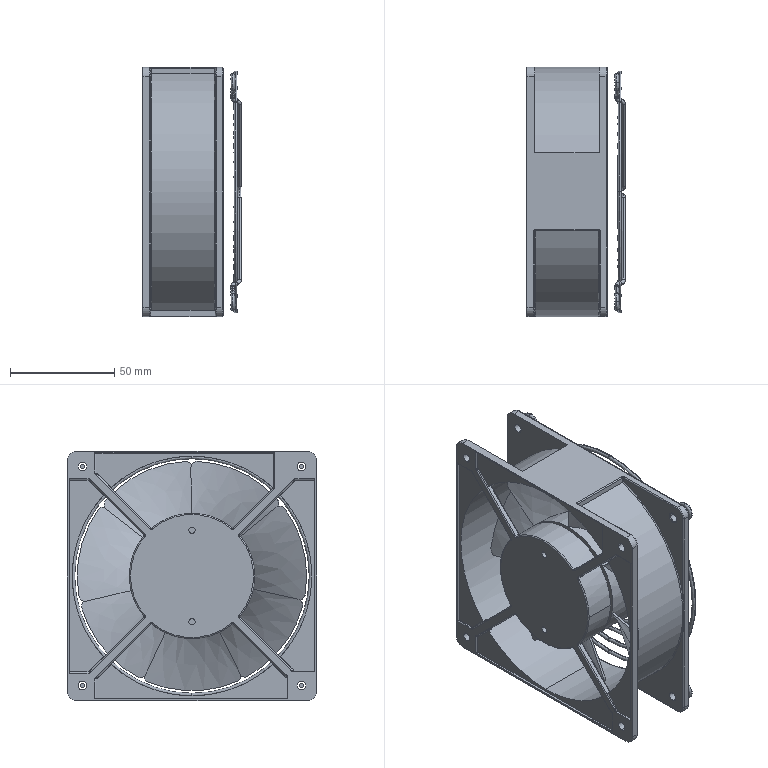Part | SolidWorks | features ICE 7, Fillet 3, CirPattern 2, Revolution 2, 3DProfileFeature 1, Extrusion 1, Helix 1, MoveCopyBody 1, Stock 1, Sweep 1 | 15 solids | 468 faces | box 47.2 x 119.523 x 119.5 mm | volume 170243 mm3 | cylinder 191 | torus 138 | plane 83 | spline 56 | commonest cylinder face diameters 1 x94 1.8 x40 4.2 x16 2 x10 6 x9 8.8 x8